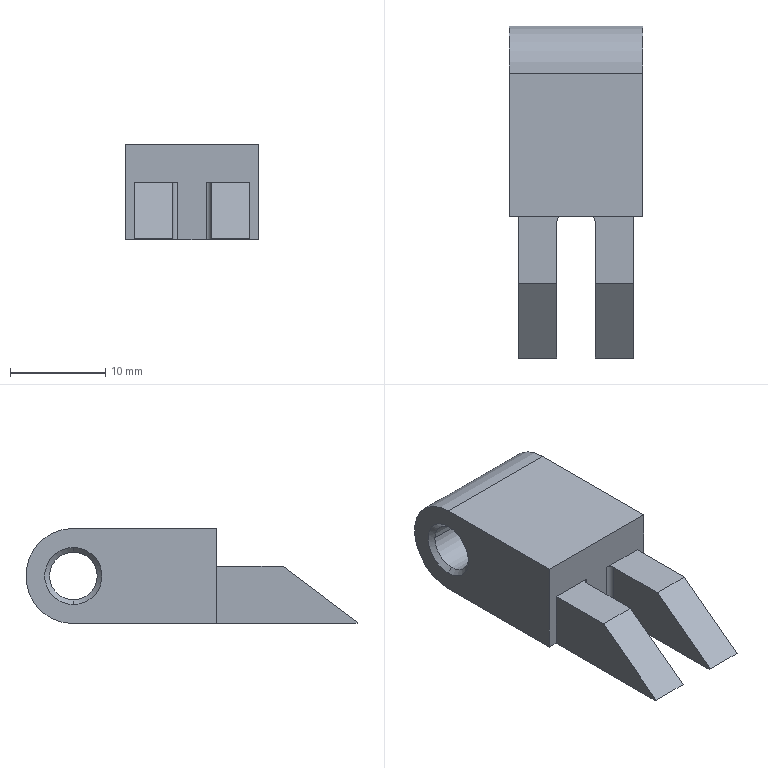Part | STEP file | PN_0011 Mount electronic clip block | 1 solid | 24 faces | box 14 x 34.832 x 10 mm | volume 2899 mm3 | plane 13 | cylinder 7 | cone 4 | commonest cylinder face diameters 1 x4 5 x2 10 x1